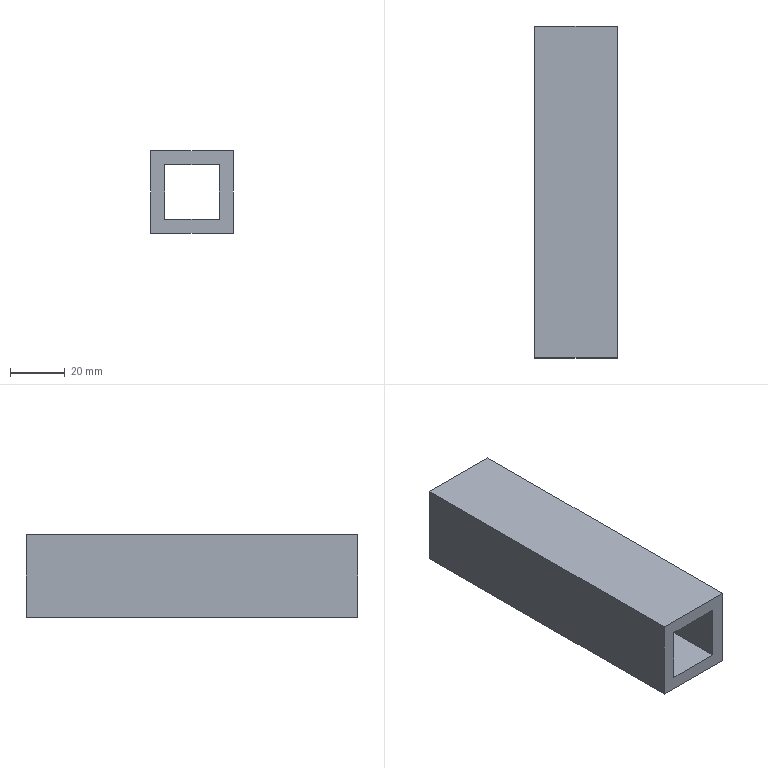Part | NX | features solid 2 | 1 solid | 10 faces | box 30 x 121 x 30 mm | volume 60500 mm3 | plane 10
STEP:
#1=CARTESIAN_POINT('',(205.,-650.,-50.));
#2=VERTEX_POINT('',#1);
#3=CARTESIAN_POINT('',(205.,-650.,-80.));
#4=VERTEX_POINT('',#3);
#5=CARTESIAN_POINT('',(205.,-650.,-80.));
#6=DIRECTION('',(0.,0.,1.));
#7=VECTOR('',#6,1000.);
#8=LINE('',#5,#7);
#9=EDGE_CURVE('',#2,#4,#8,.F.);
#10=ORIENTED_EDGE('',*,*,#9,.F.);
#11=CARTESIAN_POINT('',(175.,-650.,-50.));
#12=VERTEX_POINT('',#11);
#13=CARTESIAN_POINT('',(205.,-650.,-50.));
#14=DIRECTION('',(1.,0.,0.));
#15=VECTOR('',#14,1000.);
#16=LINE('',#13,#15);
#17=EDGE_CURVE('',#2,#12,#16,.F.);
#18=ORIENTED_EDGE('',*,*,#17,.T.);
#19=CARTESIAN_POINT('',(175.,-650.,-80.));
#20=VERTEX_POINT('',#19);
#21=CARTESIAN_POINT('',(175.,-650.,-80.));
#22=DIRECTION('',(0.,0.,-1.));
#23=VECTOR('',#22,1000.);
#24=LINE('',#21,#23);
#25=EDGE_CURVE('',#12,#20,#24,.T.);
#26=ORIENTED_EDGE('',*,*,#25,.T.);
#27=CARTESIAN_POINT('',(205.,-650.,-80.));
#28=DIRECTION('',(1.,0.,0.));
#29=VECTOR('',#28,1000.);
#30=LINE('',#27,#29);
#31=EDGE_CURVE('',#4,#20,#30,.F.);
#32=ORIENTED_EDGE('',*,*,#31,.F.);
#33=EDGE_LOOP('',(#10,#18,#26,#32));
#34=FACE_BOUND('',#33,.T.);
#35=CARTESIAN_POINT('',(200.,-650.,-55.));
#36=VERTEX_POINT('',#35);
#37=CARTESIAN_POINT('',(200.,-650.,-75.));
#38=VERTEX_POINT('',#37);
#39=CARTESIAN_POINT('',(200.,-650.,-80.));
#40=DIRECTION('',(0.,0.,1.));
#41=VECTOR('',#40,1000.);
#42=LINE('',#39,#41);
#43=EDGE_CURVE('',#36,#38,#42,.F.);
#44=ORIENTED_EDGE('',*,*,#43,.T.);
#45=CARTESIAN_POINT('',(180.,-650.,-75.));
#46=VERTEX_POINT('',#45);
#47=CARTESIAN_POINT('',(205.,-650.,-75.));
#48=DIRECTION('',(1.,0.,0.));
#49=VECTOR('',#48,1000.);
#50=LINE('',#47,#49);
#51=EDGE_CURVE('',#38,#46,#50,.F.);
#52=ORIENTED_EDGE('',*,*,#51,.T.);
#53=CARTESIAN_POINT('',(180.,-650.,-55.));
#54=VERTEX_POINT('',#53);
#55=CARTESIAN_POINT('',(180.,-650.,-80.));
#56=DIRECTION('',(0.,0.,-1.));
#57=VECTOR('',#56,1000.);
#58=LINE('',#55,#57);
#59=EDGE_CURVE('',#54,#46,#58,.T.);
#60=ORIENTED_EDGE('',*,*,#59,.F.);
#61=CARTESIAN_POINT('',(205.,-650.,-55.));
#62=DIRECTION('',(1.,0.,0.));
#63=VECTOR('',#62,1000.);
#64=LINE('',#61,#63);
#65=EDGE_CURVE('',#36,#54,#64,.F.);
#66=ORIENTED_EDGE('',*,*,#65,.F.);
#67=EDGE_LOOP('',(#44,#52,#60,#66));
#68=FACE_BOUND('',#67,.T.);
#69=CARTESIAN_POINT('',(-205.,-650.,-80.));
#70=DIRECTION('',(0.,-1.,0.));
#71=DIRECTION('',(1.,0.,0.));
#72=AXIS2_PLACEMENT_3D('',#69,#70,#71);
#73=PLANE('',#72);
#74=ADVANCED_FACE('',(#34,#68),#73,.T.);
#75=CARTESIAN_POINT('',(175.,-529.,-50.));
#76=VERTEX_POINT('',#75);
#77=CARTESIAN_POINT('',(175.,-529.,-80.));
#78=VERTEX_POINT('',#77);
#79=CARTESIAN_POINT('',(175.,-529.,-27.854));
#80=DIRECTION('',(0.,0.,-1.));
#81=VECTOR('',#80,1000.);
#82=LINE('',#79,#81);
#83=EDGE_CURVE('',#76,#78,#82,.T.);
#84=ORIENTED_EDGE('',*,*,#83,.F.);
#85=CARTESIAN_POINT('',(205.,-529.,-50.));
#86=VERTEX_POINT('',#85);
#87=CARTESIAN_POINT('',(205.,-529.,-50.));
#88=DIRECTION('',(1.,0.,0.));
#89=VECTOR('',#88,1000.);
#90=LINE('',#87,#89);
#91=EDGE_CURVE('',#86,#76,#90,.F.);
#92=ORIENTED_EDGE('',*,*,#91,.F.);
#93=CARTESIAN_POINT('',(205.,-529.,-80.));
#94=VERTEX_POINT('',#93);
#95=CARTESIAN_POINT('',(205.,-529.,-80.));
#96=DIRECTION('',(0.,0.,1.));
#97=VECTOR('',#96,1000.);
#98=LINE('',#95,#97);
#99=EDGE_CURVE('',#86,#94,#98,.F.);
#100=ORIENTED_EDGE('',*,*,#99,.T.);
#101=CARTESIAN_POINT('',(205.,-529.,-80.));
#102=DIRECTION('',(1.,0.,0.));
#103=VECTOR('',#102,1000.);
#104=LINE('',#101,#103);
#105=EDGE_CURVE('',#94,#78,#104,.F.);
#106=ORIENTED_EDGE('',*,*,#105,.T.);
#107=EDGE_LOOP('',(#84,#92,#100,#106));
#108=FACE_BOUND('',#107,.T.);
#109=CARTESIAN_POINT('',(180.,-529.,-55.));
#110=VERTEX_POINT('',#109);
#111=CARTESIAN_POINT('',(180.,-529.,-75.));
#112=VERTEX_POINT('',#111);
#113=CARTESIAN_POINT('',(180.,-529.,-27.854));
#114=DIRECTION('',(0.,0.,-1.));
#115=VECTOR('',#114,1000.);
#116=LINE('',#113,#115);
#117=EDGE_CURVE('',#110,#112,#116,.T.);
#118=ORIENTED_EDGE('',*,*,#117,.T.);
#119=CARTESIAN_POINT('',(200.,-529.,-75.));
#120=VERTEX_POINT('',#119);
#121=CARTESIAN_POINT('',(205.,-529.,-75.));
#122=DIRECTION('',(1.,0.,0.));
#123=VECTOR('',#122,1000.);
#124=LINE('',#121,#123);
#125=EDGE_CURVE('',#120,#112,#124,.F.);
#126=ORIENTED_EDGE('',*,*,#125,.F.);
#127=CARTESIAN_POINT('',(200.,-529.,-55.));
#128=VERTEX_POINT('',#127);
#129=CARTESIAN_POINT('',(200.,-529.,-80.));
#130=DIRECTION('',(0.,0.,1.));
#131=VECTOR('',#130,1000.);
#132=LINE('',#129,#131);
#133=EDGE_CURVE('',#128,#120,#132,.F.);
#134=ORIENTED_EDGE('',*,*,#133,.F.);
#135=CARTESIAN_POINT('',(205.,-529.,-55.));
#136=DIRECTION('',(1.,0.,0.));
#137=VECTOR('',#136,1000.);
#138=LINE('',#135,#137);
#139=EDGE_CURVE('',#128,#110,#138,.F.);
#140=ORIENTED_EDGE('',*,*,#139,.T.);
#141=EDGE_LOOP('',(#118,#126,#134,#140));
#142=FACE_BOUND('',#141,.T.);
#143=CARTESIAN_POINT('',(167.5,-529.,-27.854));
#144=DIRECTION('',(0.,1.,0.));
#145=DIRECTION('',(0.,0.,1.));
#146=AXIS2_PLACEMENT_3D('',#143,#144,#145);
#147=PLANE('',#146);
#148=ADVANCED_FACE('',(#108,#142),#147,.T.);
#149=ORIENTED_EDGE('',*,*,#25,.F.);
#150=CARTESIAN_POINT('',(175.,-655.,-50.));
#151=DIRECTION('',(0.,1.,0.));
#152=VECTOR('',#151,1000.);
#153=LINE('',#150,#152);
#154=EDGE_CURVE('',#12,#76,#153,.T.);
#155=ORIENTED_EDGE('',*,*,#154,.T.);
#156=ORIENTED_EDGE('',*,*,#83,.T.);
#157=CARTESIAN_POINT('',(175.,-655.,-80.));
#158=DIRECTION('',(0.,1.,0.));
#159=VECTOR('',#158,1000.);
#160=LINE('',#157,#159);
#161=EDGE_CURVE('',#20,#78,#160,.T.);
#162=ORIENTED_EDGE('',*,*,#161,.F.);
#163=EDGE_LOOP('',(#149,#155,#156,#162));
#164=FACE_BOUND('',#163,.T.);
#165=CARTESIAN_POINT('',(175.,-655.,-80.));
#166=DIRECTION('',(-1.,0.,0.));
#167=DIRECTION('',(0.,1.,0.));
#168=AXIS2_PLACEMENT_3D('',#165,#166,#167);
#169=PLANE('',#168);
#170=ADVANCED_FACE('',(#164),#169,.T.);
#171=CARTESIAN_POINT('',(205.,-655.,-50.));
#172=DIRECTION('',(0.,1.,0.));
#173=VECTOR('',#172,1000.);
#174=LINE('',#171,#173);
#175=EDGE_CURVE('',#2,#86,#174,.T.);
#176=ORIENTED_EDGE('',*,*,#175,.F.);
#177=ORIENTED_EDGE('',*,*,#9,.T.);
#178=CARTESIAN_POINT('',(205.,-655.,-80.));
#179=DIRECTION('',(0.,1.,0.));
#180=VECTOR('',#179,1000.);
#181=LINE('',#178,#180);
#182=EDGE_CURVE('',#4,#94,#181,.T.);
#183=ORIENTED_EDGE('',*,*,#182,.T.);
#184=ORIENTED_EDGE('',*,*,#99,.F.);
#185=EDGE_LOOP('',(#176,#177,#183,#184));
#186=FACE_BOUND('',#185,.T.);
#187=CARTESIAN_POINT('',(205.,-655.,-80.));
#188=DIRECTION('',(-1.,0.,0.));
#189=DIRECTION('',(0.,1.,0.));
#190=AXIS2_PLACEMENT_3D('',#187,#188,#189);
#191=PLANE('',#190);
#192=ADVANCED_FACE('',(#186),#191,.F.);
#193=ORIENTED_EDGE('',*,*,#105,.F.);
#194=ORIENTED_EDGE('',*,*,#182,.F.);
#195=ORIENTED_EDGE('',*,*,#31,.T.);
#196=ORIENTED_EDGE('',*,*,#161,.T.);
#197=EDGE_LOOP('',(#193,#194,#195,#196));
#198=FACE_BOUND('',#197,.T.);
#199=CARTESIAN_POINT('',(205.,-655.,-80.));
#200=DIRECTION('',(0.,0.,1.));
#201=DIRECTION('',(-1.,0.,0.));
#202=AXIS2_PLACEMENT_3D('',#199,#200,#201);
#203=PLANE('',#202);
#204=ADVANCED_FACE('',(#198),#203,.F.);
#205=ORIENTED_EDGE('',*,*,#91,.T.);
#206=ORIENTED_EDGE('',*,*,#154,.F.);
#207=ORIENTED_EDGE('',*,*,#17,.F.);
#208=ORIENTED_EDGE('',*,*,#175,.T.);
#209=EDGE_LOOP('',(#205,#206,#207,#208));
#210=FACE_BOUND('',#209,.T.);
#211=CARTESIAN_POINT('',(205.,-655.,-50.));
#212=DIRECTION('',(0.,0.,1.));
#213=DIRECTION('',(-1.,0.,0.));
#214=AXIS2_PLACEMENT_3D('',#211,#212,#213);
#215=PLANE('',#214);
#216=ADVANCED_FACE('',(#210),#215,.T.);
#217=ORIENTED_EDGE('',*,*,#59,.T.);
#218=CARTESIAN_POINT('',(180.,-655.,-75.));
#219=DIRECTION('',(0.,-1.,0.));
#220=VECTOR('',#219,1000.);
#221=LINE('',#218,#220);
#222=EDGE_CURVE('',#46,#112,#221,.F.);
#223=ORIENTED_EDGE('',*,*,#222,.T.);
#224=ORIENTED_EDGE('',*,*,#117,.F.);
#225=CARTESIAN_POINT('',(180.,-655.,-55.));
#226=DIRECTION('',(0.,-1.,0.));
#227=VECTOR('',#226,1000.);
#228=LINE('',#225,#227);
#229=EDGE_CURVE('',#54,#110,#228,.F.);
#230=ORIENTED_EDGE('',*,*,#229,.F.);
#231=EDGE_LOOP('',(#217,#223,#224,#230));
#232=FACE_BOUND('',#231,.T.);
#233=CARTESIAN_POINT('',(180.,-655.,-80.));
#234=DIRECTION('',(-1.,0.,0.));
#235=DIRECTION('',(0.,1.,0.));
#236=AXIS2_PLACEMENT_3D('',#233,#234,#235);
#237=PLANE('',#236);
#238=ADVANCED_FACE('',(#232),#237,.F.);
#239=CARTESIAN_POINT('',(200.,-655.,-55.));
#240=DIRECTION('',(0.,1.,0.));
#241=VECTOR('',#240,1000.);
#242=LINE('',#239,#241);
#243=EDGE_CURVE('',#36,#128,#242,.T.);
#244=ORIENTED_EDGE('',*,*,#243,.T.);
#245=ORIENTED_EDGE('',*,*,#133,.T.);
#246=CARTESIAN_POINT('',(200.,-655.,-75.));
#247=DIRECTION('',(0.,1.,0.));
#248=VECTOR('',#247,1000.);
#249=LINE('',#246,#248);
#250=EDGE_CURVE('',#38,#120,#249,.T.);
#251=ORIENTED_EDGE('',*,*,#250,.F.);
#252=ORIENTED_EDGE('',*,*,#43,.F.);
#253=EDGE_LOOP('',(#244,#245,#251,#252));
#254=FACE_BOUND('',#253,.T.);
#255=CARTESIAN_POINT('',(200.,-655.,-80.));
#256=DIRECTION('',(-1.,0.,0.));
#257=DIRECTION('',(0.,1.,0.));
#258=AXIS2_PLACEMENT_3D('',#255,#256,#257);
#259=PLANE('',#258);
#260=ADVANCED_FACE('',(#254),#259,.T.);
#261=ORIENTED_EDGE('',*,*,#125,.T.);
#262=ORIENTED_EDGE('',*,*,#222,.F.);
#263=ORIENTED_EDGE('',*,*,#51,.F.);
#264=ORIENTED_EDGE('',*,*,#250,.T.);
#265=EDGE_LOOP('',(#261,#262,#263,#264));
#266=FACE_BOUND('',#265,.T.);
#267=CARTESIAN_POINT('',(205.,-655.,-75.));
#268=DIRECTION('',(0.,0.,1.));
#269=DIRECTION('',(-1.,0.,0.));
#270=AXIS2_PLACEMENT_3D('',#267,#268,#269);
#271=PLANE('',#270);
#272=ADVANCED_FACE('',(#266),#271,.T.);
#273=ORIENTED_EDGE('',*,*,#139,.F.);
#274=ORIENTED_EDGE('',*,*,#243,.F.);
#275=ORIENTED_EDGE('',*,*,#65,.T.);
#276=ORIENTED_EDGE('',*,*,#229,.T.);
#277=EDGE_LOOP('',(#273,#274,#275,#276));
#278=FACE_BOUND('',#277,.T.);
#279=CARTESIAN_POINT('',(205.,-655.,-55.));
#280=DIRECTION('',(0.,0.,1.));
#281=DIRECTION('',(-1.,0.,0.));
#282=AXIS2_PLACEMENT_3D('',#279,#280,#281);
#283=PLANE('',#282);
#284=ADVANCED_FACE('',(#278),#283,.F.);
#285=CLOSED_SHELL('',(#74,#148,#170,#192,#204,#216,#238,#260,#272,#284));
#286=MANIFOLD_SOLID_BREP('',#285);
#287=(LENGTH_UNIT()NAMED_UNIT(*)SI_UNIT(.MILLI.,.METRE.));
#288=UNCERTAINTY_MEASURE_WITH_UNIT(LENGTH_MEASURE(0.00001),#287,'','');
#289=(NAMED_UNIT(*)PLANE_ANGLE_UNIT()SI_UNIT($,.RADIAN.));
#290=(NAMED_UNIT(*)SI_UNIT($,.STERADIAN.)SOLID_ANGLE_UNIT());
#291=(GEOMETRIC_REPRESENTATION_CONTEXT(3)GLOBAL_UNCERTAINTY_ASSIGNED_CONTEXT((#288))GLOBAL_UNIT_ASSIGNED_CONTEXT((#287,#289,#290))REPRESENTATION_CONTEXT('',''));
#292=ADVANCED_BREP_SHAPE_REPRESENTATION('',(#286),#291);